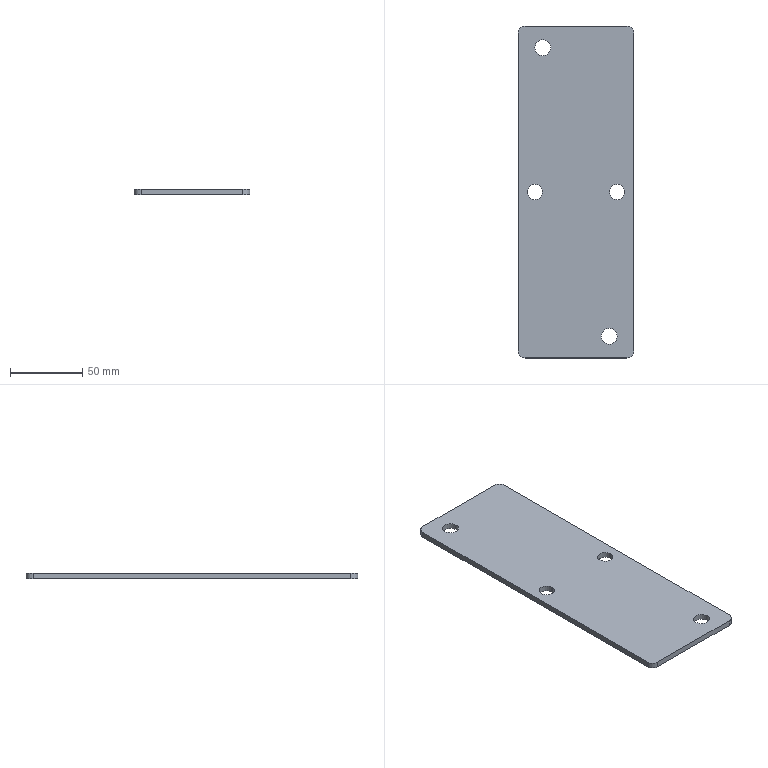Part | STEP file | 1_id78_x_t | 1 solid | 16 faces | box 80 x 230 x 4 mm | volume 72058 mm3 | cylinder 10 | plane 6 | commonest cylinder face diameters 10 x4 10.524 x4 11 x2
STEP:
#1=CARTESIAN_POINT('',(0.,0.,0.));
#2=DIRECTION('',(0.,0.,1.));
#3=DIRECTION('',(1.,0.,0.));
#4=AXIS2_PLACEMENT_3D('',#1,#2,#3);
#5=CARTESIAN_POINT('',(430.488,177.5,-105.));
#6=VERTEX_POINT('',#5);
#7=CARTESIAN_POINT('',(441.012,177.5,-105.));
#8=VERTEX_POINT('',#7);
#9=CARTESIAN_POINT('',(435.75,177.5,-105.));
#10=DIRECTION('',(0.,0.,1.));
#11=DIRECTION('',(1.,0.,0.));
#12=AXIS2_PLACEMENT_3D('',#9,#10,#11);
#13=CIRCLE('',#12,5.262);
#14=CARTESIAN_POINT('',(435.75,177.5,-101.));
#15=DIRECTION('',(0.,0.,1.));
#16=DIRECTION('',(1.,0.,0.));
#17=AXIS2_PLACEMENT_3D('',#14,#15,#16);
#18=CYLINDRICAL_SURFACE('',#17,5.262);
#19=CARTESIAN_POINT('',(0.,-4.));
#20=DIRECTION('',(1.,0.));
#21=VECTOR('',#20,1.);
#22=LINE('',#19,#21);
#23=(GEOMETRIC_REPRESENTATION_CONTEXT(2)PARAMETRIC_REPRESENTATION_CONTEXT()REPRESENTATION_CONTEXT('',''));
#24=DEFINITIONAL_REPRESENTATION('',(#22),#23);
#25=PCURVE('',#18,#24);
#26=CARTESIAN_POINT('',(272.727,177.5,-105.));
#27=DIRECTION('',(0.,0.,1.));
#28=DIRECTION('',(-1.,0.,0.));
#29=AXIS2_PLACEMENT_3D('',#26,#27,#28);
#30=PLANE('',#29);
#31=CARTESIAN_POINT('',(-163.023,-0.000000031));
#32=DIRECTION('',(-1.,0.));
#33=AXIS2_PLACEMENT_2D('',#31,#32);
#34=CIRCLE('',#33,5.262);
#35=(GEOMETRIC_REPRESENTATION_CONTEXT(2)PARAMETRIC_REPRESENTATION_CONTEXT()REPRESENTATION_CONTEXT('',''));
#36=DEFINITIONAL_REPRESENTATION('',(#34),#35);
#37=PCURVE('',#30,#36);
#38=SURFACE_CURVE('',#13,(#25,#37),.PCURVE_S1.);
#39=EDGE_CURVE('',#6,#8,#38,.T.);
#40=ORIENTED_EDGE('',*,*,#39,.T.);
#41=CARTESIAN_POINT('',(441.012,177.5,-101.));
#42=VERTEX_POINT('',#41);
#43=CARTESIAN_POINT('',(441.012,177.5,-101.));
#44=DIRECTION('',(0.,0.,1.));
#45=VECTOR('',#44,1.);
#46=LINE('',#43,#45);
#47=CARTESIAN_POINT('',(6.283,0.));
#48=DIRECTION('',(0.,1.));
#49=VECTOR('',#48,1.);
#50=LINE('',#47,#49);
#51=(GEOMETRIC_REPRESENTATION_CONTEXT(2)PARAMETRIC_REPRESENTATION_CONTEXT()REPRESENTATION_CONTEXT('',''));
#52=DEFINITIONAL_REPRESENTATION('',(#50),#51);
#53=PCURVE('',#18,#52);
#54=CARTESIAN_POINT('',(435.75,177.5,-101.));
#55=DIRECTION('',(0.,0.,1.));
#56=DIRECTION('',(1.,0.,0.));
#57=AXIS2_PLACEMENT_3D('',#54,#55,#56);
#58=CYLINDRICAL_SURFACE('',#57,5.262);
#59=CARTESIAN_POINT('',(0.000004723,0.));
#60=DIRECTION('',(0.,1.));
#61=VECTOR('',#60,1.);
#62=LINE('',#59,#61);
#63=(GEOMETRIC_REPRESENTATION_CONTEXT(2)PARAMETRIC_REPRESENTATION_CONTEXT()REPRESENTATION_CONTEXT('',''));
#64=DEFINITIONAL_REPRESENTATION('',(#62),#63);
#65=PCURVE('',#58,#64);
#66=SURFACE_CURVE('',#46,(#53,#65),.PCURVE_S1.);
#67=EDGE_CURVE('',#8,#42,#66,.T.);
#68=ORIENTED_EDGE('',*,*,#67,.T.);
#69=CARTESIAN_POINT('',(430.488,177.5,-101.));
#70=VERTEX_POINT('',#69);
#71=CARTESIAN_POINT('',(435.75,177.5,-101.));
#72=DIRECTION('',(0.,0.,1.));
#73=DIRECTION('',(1.,0.,0.));
#74=AXIS2_PLACEMENT_3D('',#71,#72,#73);
#75=CIRCLE('',#74,5.262);
#76=CARTESIAN_POINT('',(0.,0.));
#77=DIRECTION('',(1.,0.));
#78=VECTOR('',#77,1.);
#79=LINE('',#76,#78);
#80=(GEOMETRIC_REPRESENTATION_CONTEXT(2)PARAMETRIC_REPRESENTATION_CONTEXT()REPRESENTATION_CONTEXT('',''));
#81=DEFINITIONAL_REPRESENTATION('',(#79),#80);
#82=PCURVE('',#18,#81);
#83=CARTESIAN_POINT('',(272.727,177.5,-101.));
#84=DIRECTION('',(0.,0.,1.));
#85=DIRECTION('',(-1.,0.,0.));
#86=AXIS2_PLACEMENT_3D('',#83,#84,#85);
#87=PLANE('',#86);
#88=CARTESIAN_POINT('',(-163.023,-0.000000031));
#89=DIRECTION('',(-1.,0.));
#90=AXIS2_PLACEMENT_2D('',#88,#89);
#91=CIRCLE('',#90,5.262);
#92=(GEOMETRIC_REPRESENTATION_CONTEXT(2)PARAMETRIC_REPRESENTATION_CONTEXT()REPRESENTATION_CONTEXT('',''));
#93=DEFINITIONAL_REPRESENTATION('',(#91),#92);
#94=PCURVE('',#87,#93);
#95=SURFACE_CURVE('',#75,(#82,#94),.PCURVE_S1.);
#96=EDGE_CURVE('',#70,#42,#95,.T.);
#97=ORIENTED_EDGE('',*,*,#96,.F.);
#98=CARTESIAN_POINT('',(430.488,177.5,-101.));
#99=DIRECTION('',(0.,0.,-1.));
#100=VECTOR('',#99,1.);
#101=LINE('',#98,#100);
#102=CARTESIAN_POINT('',(3.142,0.));
#103=DIRECTION('',(0.,-1.));
#104=VECTOR('',#103,1.);
#105=LINE('',#102,#104);
#106=(GEOMETRIC_REPRESENTATION_CONTEXT(2)PARAMETRIC_REPRESENTATION_CONTEXT()REPRESENTATION_CONTEXT('',''));
#107=DEFINITIONAL_REPRESENTATION('',(#105),#106);
#108=PCURVE('',#18,#107);
#109=CARTESIAN_POINT('',(3.142,0.));
#110=DIRECTION('',(0.,-1.));
#111=VECTOR('',#110,1.);
#112=LINE('',#109,#111);
#113=(GEOMETRIC_REPRESENTATION_CONTEXT(2)PARAMETRIC_REPRESENTATION_CONTEXT()REPRESENTATION_CONTEXT('',''));
#114=DEFINITIONAL_REPRESENTATION('',(#112),#113);
#115=PCURVE('',#58,#114);
#116=SURFACE_CURVE('',#101,(#108,#115),.PCURVE_S1.);
#117=EDGE_CURVE('',#70,#6,#116,.T.);
#118=ORIENTED_EDGE('',*,*,#117,.T.);
#119=EDGE_LOOP('',(#40,#68,#97,#118));
#120=FACE_BOUND('',#119,.F.);
#121=ADVANCED_FACE('',(#120),#18,.F.);
#122=CARTESIAN_POINT('',(498.162,177.5,-105.));
#123=VERTEX_POINT('',#122);
#124=CARTESIAN_POINT('',(487.638,177.5,-105.));
#125=VERTEX_POINT('',#124);
#126=CARTESIAN_POINT('',(492.9,177.5,-105.));
#127=DIRECTION('',(0.,0.,1.));
#128=DIRECTION('',(1.,0.,0.));
#129=AXIS2_PLACEMENT_3D('',#126,#127,#128);
#130=CIRCLE('',#129,5.262);
#131=CARTESIAN_POINT('',(492.9,177.5,-101.));
#132=DIRECTION('',(0.,0.,1.));
#133=DIRECTION('',(1.,0.,0.));
#134=AXIS2_PLACEMENT_3D('',#131,#132,#133);
#135=CYLINDRICAL_SURFACE('',#134,5.262);
#136=CARTESIAN_POINT('',(0.,-4.));
#137=DIRECTION('',(1.,0.));
#138=VECTOR('',#137,1.);
#139=LINE('',#136,#138);
#140=(GEOMETRIC_REPRESENTATION_CONTEXT(2)PARAMETRIC_REPRESENTATION_CONTEXT()REPRESENTATION_CONTEXT('',''));
#141=DEFINITIONAL_REPRESENTATION('',(#139),#140);
#142=PCURVE('',#135,#141);
#143=CARTESIAN_POINT('',(-220.173,0.00003309));
#144=DIRECTION('',(-1.,0.));
#145=AXIS2_PLACEMENT_2D('',#143,#144);
#146=CIRCLE('',#145,5.262);
#147=(GEOMETRIC_REPRESENTATION_CONTEXT(2)PARAMETRIC_REPRESENTATION_CONTEXT()REPRESENTATION_CONTEXT('',''));
#148=DEFINITIONAL_REPRESENTATION('',(#146),#147);
#149=PCURVE('',#30,#148);
#150=SURFACE_CURVE('',#130,(#142,#149),.PCURVE_S1.);
#151=EDGE_CURVE('',#123,#125,#150,.T.);
#152=ORIENTED_EDGE('',*,*,#151,.T.);
#153=CARTESIAN_POINT('',(487.638,177.5,-101.));
#154=VERTEX_POINT('',#153);
#155=CARTESIAN_POINT('',(487.638,177.5,-101.));
#156=DIRECTION('',(0.,0.,1.));
#157=VECTOR('',#156,1.);
#158=LINE('',#155,#157);
#159=CARTESIAN_POINT('',(3.142,0.));
#160=DIRECTION('',(0.,1.));
#161=VECTOR('',#160,1.);
#162=LINE('',#159,#161);
#163=(GEOMETRIC_REPRESENTATION_CONTEXT(2)PARAMETRIC_REPRESENTATION_CONTEXT()REPRESENTATION_CONTEXT('',''));
#164=DEFINITIONAL_REPRESENTATION('',(#162),#163);
#165=PCURVE('',#135,#164);
#166=CARTESIAN_POINT('',(492.9,177.5,-101.));
#167=DIRECTION('',(0.,0.,1.));
#168=DIRECTION('',(1.,0.,0.));
#169=AXIS2_PLACEMENT_3D('',#166,#167,#168);
#170=CYLINDRICAL_SURFACE('',#169,5.262);
#171=CARTESIAN_POINT('',(3.142,0.));
#172=DIRECTION('',(0.,1.));
#173=VECTOR('',#172,1.);
#174=LINE('',#171,#173);
#175=(GEOMETRIC_REPRESENTATION_CONTEXT(2)PARAMETRIC_REPRESENTATION_CONTEXT()REPRESENTATION_CONTEXT('',''));
#176=DEFINITIONAL_REPRESENTATION('',(#174),#175);
#177=PCURVE('',#170,#176);
#178=SURFACE_CURVE('',#158,(#165,#177),.PCURVE_S1.);
#179=EDGE_CURVE('',#125,#154,#178,.T.);
#180=ORIENTED_EDGE('',*,*,#179,.T.);
#181=CARTESIAN_POINT('',(498.162,177.5,-101.));
#182=VERTEX_POINT('',#181);
#183=CARTESIAN_POINT('',(492.9,177.5,-101.));
#184=DIRECTION('',(0.,0.,1.));
#185=DIRECTION('',(1.,0.,0.));
#186=AXIS2_PLACEMENT_3D('',#183,#184,#185);
#187=CIRCLE('',#186,5.262);
#188=CARTESIAN_POINT('',(0.,0.));
#189=DIRECTION('',(1.,0.));
#190=VECTOR('',#189,1.);
#191=LINE('',#188,#190);
#192=(GEOMETRIC_REPRESENTATION_CONTEXT(2)PARAMETRIC_REPRESENTATION_CONTEXT()REPRESENTATION_CONTEXT('',''));
#193=DEFINITIONAL_REPRESENTATION('',(#191),#192);
#194=PCURVE('',#135,#193);
#195=CARTESIAN_POINT('',(-220.173,0.00003309));
#196=DIRECTION('',(-1.,0.));
#197=AXIS2_PLACEMENT_2D('',#195,#196);
#198=CIRCLE('',#197,5.262);
#199=(GEOMETRIC_REPRESENTATION_CONTEXT(2)PARAMETRIC_REPRESENTATION_CONTEXT()REPRESENTATION_CONTEXT('',''));
#200=DEFINITIONAL_REPRESENTATION('',(#198),#199);
#201=PCURVE('',#87,#200);
#202=SURFACE_CURVE('',#187,(#194,#201),.PCURVE_S1.);
#203=EDGE_CURVE('',#182,#154,#202,.T.);
#204=ORIENTED_EDGE('',*,*,#203,.F.);
#205=CARTESIAN_POINT('',(498.162,177.5,-101.));
#206=DIRECTION('',(0.,0.,-1.));
#207=VECTOR('',#206,1.);
#208=LINE('',#205,#207);
#209=CARTESIAN_POINT('',(0.000004723,0.));
#210=DIRECTION('',(0.,-1.));
#211=VECTOR('',#210,1.);
#212=LINE('',#209,#211);
#213=(GEOMETRIC_REPRESENTATION_CONTEXT(2)PARAMETRIC_REPRESENTATION_CONTEXT()REPRESENTATION_CONTEXT('',''));
#214=DEFINITIONAL_REPRESENTATION('',(#212),#213);
#215=PCURVE('',#135,#214);
#216=CARTESIAN_POINT('',(6.283,0.));
#217=DIRECTION('',(0.,-1.));
#218=VECTOR('',#217,1.);
#219=LINE('',#216,#218);
#220=(GEOMETRIC_REPRESENTATION_CONTEXT(2)PARAMETRIC_REPRESENTATION_CONTEXT()REPRESENTATION_CONTEXT('',''));
#221=DEFINITIONAL_REPRESENTATION('',(#219),#220);
#222=PCURVE('',#170,#221);
#223=SURFACE_CURVE('',#208,(#215,#222),.PCURVE_S1.);
#224=EDGE_CURVE('',#182,#123,#223,.T.);
#225=ORIENTED_EDGE('',*,*,#224,.T.);
#226=EDGE_LOOP('',(#152,#180,#204,#225));
#227=FACE_BOUND('',#226,.F.);
#228=ADVANCED_FACE('',(#227),#135,.F.);
#229=CARTESIAN_POINT('',(499.325,292.5,-101.));
#230=VERTEX_POINT('',#229);
#231=CARTESIAN_POINT('',(499.325,292.5,-105.));
#232=VERTEX_POINT('',#231);
#233=CARTESIAN_POINT('',(499.325,292.5,-101.));
#234=DIRECTION('',(0.,0.,-1.));
#235=VECTOR('',#234,1.);
#236=LINE('',#233,#235);
#237=CARTESIAN_POINT('',(499.325,287.5,-101.));
#238=DIRECTION('',(0.,0.,-1.));
#239=DIRECTION('',(-1.,0.,0.));
#240=AXIS2_PLACEMENT_3D('',#237,#238,#239);
#241=CYLINDRICAL_SURFACE('',#240,5.);
#242=CARTESIAN_POINT('',(1.571,0.));
#243=DIRECTION('',(0.,1.));
#244=VECTOR('',#243,1.);
#245=LINE('',#242,#244);
#246=(GEOMETRIC_REPRESENTATION_CONTEXT(2)PARAMETRIC_REPRESENTATION_CONTEXT()REPRESENTATION_CONTEXT('',''));
#247=DEFINITIONAL_REPRESENTATION('',(#245),#246);
#248=PCURVE('',#241,#247);
#249=CARTESIAN_POINT('',(272.727,292.5,-101.));
#250=DIRECTION('',(0.,1.,0.));
#251=DIRECTION('',(-1.,0.,0.));
#252=AXIS2_PLACEMENT_3D('',#249,#250,#251);
#253=PLANE('',#252);
#254=CARTESIAN_POINT('',(-226.598,0.));
#255=DIRECTION('',(0.,-1.));
#256=VECTOR('',#255,1.);
#257=LINE('',#254,#256);
#258=(GEOMETRIC_REPRESENTATION_CONTEXT(2)PARAMETRIC_REPRESENTATION_CONTEXT()REPRESENTATION_CONTEXT('',''));
#259=DEFINITIONAL_REPRESENTATION('',(#257),#258);
#260=PCURVE('',#253,#259);
#261=SURFACE_CURVE('',#236,(#248,#260),.PCURVE_S1.);
#262=EDGE_CURVE('',#230,#232,#261,.T.);
#263=ORIENTED_EDGE('',*,*,#262,.F.);
#264=CARTESIAN_POINT('',(504.325,287.5,-101.));
#265=VERTEX_POINT('',#264);
#266=CARTESIAN_POINT('',(499.325,287.5,-101.));
#267=DIRECTION('',(0.,0.,-1.));
#268=DIRECTION('',(-1.,0.,0.));
#269=AXIS2_PLACEMENT_3D('',#266,#267,#268);
#270=CIRCLE('',#269,5.);
#271=CARTESIAN_POINT('',(0.,0.));
#272=DIRECTION('',(1.,0.));
#273=VECTOR('',#272,1.);
#274=LINE('',#271,#273);
#275=(GEOMETRIC_REPRESENTATION_CONTEXT(2)PARAMETRIC_REPRESENTATION_CONTEXT()REPRESENTATION_CONTEXT('',''));
#276=DEFINITIONAL_REPRESENTATION('',(#274),#275);
#277=PCURVE('',#241,#276);
#278=CARTESIAN_POINT('',(-221.598,-110.));
#279=CARTESIAN_POINT('',(-221.598,-118.66));
#280=CARTESIAN_POINT('',(-229.098,-114.33));
#281=CARTESIAN_POINT('',(-236.598,-110.));
#282=CARTESIAN_POINT('',(-229.098,-105.67));
#283=CARTESIAN_POINT('',(-221.598,-101.34));
#284=CARTESIAN_POINT('',(-221.598,-110.));
#285=(BOUNDED_CURVE()B_SPLINE_CURVE(2,(#278,#279,#280,#281,#282,#283,#284),.UNSPECIFIED.,.T.,.F.)B_SPLINE_CURVE_WITH_KNOTS((1,2,2,2,2,1),(-2.094,0.,2.094,4.189,6.283,8.378),.UNSPECIFIED.)CURVE()GEOMETRIC_REPRESENTATION_ITEM()RATIONAL_B_SPLINE_CURVE((1.,0.5,1.,0.5,1.,0.5,1.))REPRESENTATION_ITEM(''));
#286=(GEOMETRIC_REPRESENTATION_CONTEXT(2)PARAMETRIC_REPRESENTATION_CONTEXT()REPRESENTATION_CONTEXT('',''));
#287=DEFINITIONAL_REPRESENTATION('',(#285),#286);
#288=PCURVE('',#87,#287);
#289=SURFACE_CURVE('',#270,(#277,#288),.PCURVE_S1.);
#290=EDGE_CURVE('',#230,#265,#289,.T.);
#291=ORIENTED_EDGE('',*,*,#290,.T.);
#292=CARTESIAN_POINT('',(504.325,287.5,-105.));
#293=VERTEX_POINT('',#292);
#294=CARTESIAN_POINT('',(504.325,287.5,-101.));
#295=DIRECTION('',(0.,0.,-1.));
#296=VECTOR('',#295,1.);
#297=LINE('',#294,#296);
#298=CARTESIAN_POINT('',(3.142,0.));
#299=DIRECTION('',(0.,1.));
#300=VECTOR('',#299,1.);
#301=LINE('',#298,#300);
#302=(GEOMETRIC_REPRESENTATION_CONTEXT(2)PARAMETRIC_REPRESENTATION_CONTEXT()REPRESENTATION_CONTEXT('',''));
#303=DEFINITIONAL_REPRESENTATION('',(#301),#302);
#304=PCURVE('',#241,#303);
#305=CARTESIAN_POINT('',(504.325,177.5,-101.));
#306=DIRECTION('',(-1.,0.,0.));
#307=DIRECTION('',(0.,-1.,0.));
#308=AXIS2_PLACEMENT_3D('',#305,#306,#307);
#309=PLANE('',#308);
#310=CARTESIAN_POINT('',(-110.,0.));
#311=DIRECTION('',(0.,-1.));
#312=VECTOR('',#311,1.);
#313=LINE('',#310,#312);
#314=(GEOMETRIC_REPRESENTATION_CONTEXT(2)PARAMETRIC_REPRESENTATION_CONTEXT()REPRESENTATION_CONTEXT('',''));
#315=DEFINITIONAL_REPRESENTATION('',(#313),#314);
#316=PCURVE('',#309,#315);
#317=SURFACE_CURVE('',#297,(#304,#316),.PCURVE_S1.);
#318=EDGE_CURVE('',#265,#293,#317,.T.);
#319=ORIENTED_EDGE('',*,*,#318,.T.);
#320=CARTESIAN_POINT('',(499.325,287.5,-105.));
#321=DIRECTION('',(0.,0.,-1.));
#322=DIRECTION('',(-1.,0.,0.));
#323=AXIS2_PLACEMENT_3D('',#320,#321,#322);
#324=CIRCLE('',#323,5.);
#325=CARTESIAN_POINT('',(0.,4.));
#326=DIRECTION('',(1.,0.));
#327=VECTOR('',#326,1.);
#328=LINE('',#325,#327);
#329=(GEOMETRIC_REPRESENTATION_CONTEXT(2)PARAMETRIC_REPRESENTATION_CONTEXT()REPRESENTATION_CONTEXT('',''));
#330=DEFINITIONAL_REPRESENTATION('',(#328),#329);
#331=PCURVE('',#241,#330);
#332=CARTESIAN_POINT('',(-221.598,-110.));
#333=CARTESIAN_POINT('',(-221.598,-118.66));
#334=CARTESIAN_POINT('',(-229.098,-114.33));
#335=CARTESIAN_POINT('',(-236.598,-110.));
#336=CARTESIAN_POINT('',(-229.098,-105.67));
#337=CARTESIAN_POINT('',(-221.598,-101.34));
#338=CARTESIAN_POINT('',(-221.598,-110.));
#339=(BOUNDED_CURVE()B_SPLINE_CURVE(2,(#332,#333,#334,#335,#336,#337,#338),.UNSPECIFIED.,.T.,.F.)B_SPLINE_CURVE_WITH_KNOTS((1,2,2,2,2,1),(-2.094,0.,2.094,4.189,6.283,8.378),.UNSPECIFIED.)CURVE()GEOMETRIC_REPRESENTATION_ITEM()RATIONAL_B_SPLINE_CURVE((1.,0.5,1.,0.5,1.,0.5,1.))REPRESENTATION_ITEM(''));
#340=(GEOMETRIC_REPRESENTATION_CONTEXT(2)PARAMETRIC_REPRESENTATION_CONTEXT()REPRESENTATION_CONTEXT('',''));
#341=DEFINITIONAL_REPRESENTATION('',(#339),#340);
#342=PCURVE('',#30,#341);
#343=SURFACE_CURVE('',#324,(#331,#342),.PCURVE_S1.);
#344=EDGE_CURVE('',#232,#293,#343,.T.);
#345=ORIENTED_EDGE('',*,*,#344,.F.);
#346=EDGE_LOOP('',(#263,#291,#319,#345));
#347=FACE_BOUND('',#346,.T.);
#348=ADVANCED_FACE('',(#347),#241,.T.);
#349=ORIENTED_EDGE('',*,*,#318,.F.);
#350=CARTESIAN_POINT('',(504.325,67.5,-101.));
#351=VERTEX_POINT('',#350);
#352=CARTESIAN_POINT('',(504.325,177.5,-101.));
#353=DIRECTION('',(0.,1.,0.));
#354=VECTOR('',#353,1.);
#355=LINE('',#352,#354);
#356=CARTESIAN_POINT('',(0.,0.));
#357=DIRECTION('',(-1.,0.));
#358=VECTOR('',#357,1.);
#359=LINE('',#356,#358);
#360=(GEOMETRIC_REPRESENTATION_CONTEXT(2)PARAMETRIC_REPRESENTATION_CONTEXT()REPRESENTATION_CONTEXT('',''));
#361=DEFINITIONAL_REPRESENTATION('',(#359),#360);
#362=PCURVE('',#309,#361);
#363=CARTESIAN_POINT('',(-231.598,0.));
#364=DIRECTION('',(0.,-1.));
#365=VECTOR('',#364,1.);
#366=LINE('',#363,#365);
#367=(GEOMETRIC_REPRESENTATION_CONTEXT(2)PARAMETRIC_REPRESENTATION_CONTEXT()REPRESENTATION_CONTEXT('',''));
#368=DEFINITIONAL_REPRESENTATION('',(#366),#367);
#369=PCURVE('',#87,#368);
#370=SURFACE_CURVE('',#355,(#362,#369),.PCURVE_S1.);
#371=EDGE_CURVE('',#351,#265,#370,.T.);
#372=ORIENTED_EDGE('',*,*,#371,.F.);
#373=CARTESIAN_POINT('',(504.325,67.5,-105.));
#374=VERTEX_POINT('',#373);
#375=CARTESIAN_POINT('',(504.325,67.5,-101.));
#376=DIRECTION('',(0.,0.,-1.));
#377=VECTOR('',#376,1.);
#378=LINE('',#375,#377);
#379=CARTESIAN_POINT('',(110.,0.));
#380=DIRECTION('',(0.,-1.));
#381=VECTOR('',#380,1.);
#382=LINE('',#379,#381);
#383=(GEOMETRIC_REPRESENTATION_CONTEXT(2)PARAMETRIC_REPRESENTATION_CONTEXT()REPRESENTATION_CONTEXT('',''));
#384=DEFINITIONAL_REPRESENTATION('',(#382),#383);
#385=PCURVE('',#309,#384);
#386=CARTESIAN_POINT('',(499.325,67.5,-101.));
#387=DIRECTION('',(0.,0.,-1.));
#388=DIRECTION('',(-1.,0.,0.));
#389=AXIS2_PLACEMENT_3D('',#386,#387,#388);
#390=CYLINDRICAL_SURFACE('',#389,5.);
#391=CARTESIAN_POINT('',(3.142,0.));
#392=DIRECTION('',(0.,1.));
#393=VECTOR('',#392,1.);
#394=LINE('',#391,#393);
#395=(GEOMETRIC_REPRESENTATION_CONTEXT(2)PARAMETRIC_REPRESENTATION_CONTEXT()REPRESENTATION_CONTEXT('',''));
#396=DEFINITIONAL_REPRESENTATION('',(#394),#395);
#397=PCURVE('',#390,#396);
#398=SURFACE_CURVE('',#378,(#385,#397),.PCURVE_S1.);
#399=EDGE_CURVE('',#351,#374,#398,.T.);
#400=ORIENTED_EDGE('',*,*,#399,.T.);
#401=CARTESIAN_POINT('',(504.325,177.5,-105.));
#402=DIRECTION('',(0.,1.,0.));
#403=VECTOR('',#402,1.);
#404=LINE('',#401,#403);
#405=CARTESIAN_POINT('',(0.,-4.));
#406=DIRECTION('',(-1.,0.));
#407=VECTOR('',#406,1.);
#408=LINE('',#405,#407);
#409=(GEOMETRIC_REPRESENTATION_CONTEXT(2)PARAMETRIC_REPRESENTATION_CONTEXT()REPRESENTATION_CONTEXT('',''));
#410=DEFINITIONAL_REPRESENTATION('',(#408),#409);
#411=PCURVE('',#309,#410);
#412=CARTESIAN_POINT('',(-231.598,0.));
#413=DIRECTION('',(0.,-1.));
#414=VECTOR('',#413,1.);
#415=LINE('',#412,#414);
#416=(GEOMETRIC_REPRESENTATION_CONTEXT(2)PARAMETRIC_REPRESENTATION_CONTEXT()REPRESENTATION_CONTEXT('',''));
#417=DEFINITIONAL_REPRESENTATION('',(#415),#416);
#418=PCURVE('',#30,#417);
#419=SURFACE_CURVE('',#404,(#411,#418),.PCURVE_S1.);
#420=EDGE_CURVE('',#374,#293,#419,.T.);
#421=ORIENTED_EDGE('',*,*,#420,.T.);
#422=EDGE_LOOP('',(#349,#372,#400,#421));
#423=FACE_BOUND('',#422,.T.);
#424=ADVANCED_FACE('',(#423),#309,.F.);
#425=ORIENTED_EDGE('',*,*,#399,.F.);
#426=CARTESIAN_POINT('',(499.325,62.5,-101.));
#427=VERTEX_POINT('',#426);
#428=CARTESIAN_POINT('',(499.325,67.5,-101.));
#429=DIRECTION('',(0.,0.,-1.));
#430=DIRECTION('',(-1.,0.,0.));
#431=AXIS2_PLACEMENT_3D('',#428,#429,#430);
#432=CIRCLE('',#431,5.);
#433=CARTESIAN_POINT('',(0.,0.));
#434=DIRECTION('',(1.,0.));
#435=VECTOR('',#434,1.);
#436=LINE('',#433,#435);
#437=(GEOMETRIC_REPRESENTATION_CONTEXT(2)PARAMETRIC_REPRESENTATION_CONTEXT()REPRESENTATION_CONTEXT('',''));
#438=DEFINITIONAL_REPRESENTATION('',(#436),#437);
#439=PCURVE('',#390,#438);
#440=CARTESIAN_POINT('',(-221.598,110.));
#441=CARTESIAN_POINT('',(-221.598,101.34));
#442=CARTESIAN_POINT('',(-229.098,105.67));
#443=CARTESIAN_POINT('',(-236.598,110.));
#444=CARTESIAN_POINT('',(-229.098,114.33));
#445=CARTESIAN_POINT('',(-221.598,118.66));
#446=CARTESIAN_POINT('',(-221.598,110.));
#447=(BOUNDED_CURVE()B_SPLINE_CURVE(2,(#440,#441,#442,#443,#444,#445,#446),.UNSPECIFIED.,.T.,.F.)B_SPLINE_CURVE_WITH_KNOTS((1,2,2,2,2,1),(-2.094,0.,2.094,4.189,6.283,8.378),.UNSPECIFIED.)CURVE()GEOMETRIC_REPRESENTATION_ITEM()RATIONAL_B_SPLINE_CURVE((1.,0.5,1.,0.5,1.,0.5,1.))REPRESENTATION_ITEM(''));
#448=(GEOMETRIC_REPRESENTATION_CONTEXT(2)PARAMETRIC_REPRESENTATION_CONTEXT()REPRESENTATION_CONTEXT('',''));
#449=DEFINITIONAL_REPRESENTATION('',(#447),#448);
#450=PCURVE('',#87,#449);
#451=SURFACE_CURVE('',#432,(#439,#450),.PCURVE_S1.);
#452=EDGE_CURVE('',#351,#427,#451,.T.);
#453=ORIENTED_EDGE('',*,*,#452,.T.);
#454=CARTESIAN_POINT('',(499.325,62.5,-105.));
#455=VERTEX_POINT('',#454);
#456=CARTESIAN_POINT('',(499.325,62.5,-101.));
#457=DIRECTION('',(0.,0.,-1.));
#458=VECTOR('',#457,1.);
#459=LINE('',#456,#458);
#460=CARTESIAN_POINT('',(4.712,0.));
#461=DIRECTION('',(0.,1.));
#462=VECTOR('',#461,1.);
#463=LINE('',#460,#462);
#464=(GEOMETRIC_REPRESENTATION_CONTEXT(2)PARAMETRIC_REPRESENTATION_CONTEXT()REPRESENTATION_CONTEXT('',''));
#465=DEFINITIONAL_REPRESENTATION('',(#463),#464);
#466=PCURVE('',#390,#465);
#467=CARTESIAN_POINT('',(272.727,62.5,-101.));
#468=DIRECTION('',(0.,1.,0.));
#469=DIRECTION('',(-1.,0.,0.));
#470=AXIS2_PLACEMENT_3D('',#467,#468,#469);
#471=PLANE('',#470);
#472=CARTESIAN_POINT('',(-226.598,0.));
#473=DIRECTION('',(0.,-1.));
#474=VECTOR('',#473,1.);
#475=LINE('',#472,#474);
#476=(GEOMETRIC_REPRESENTATION_CONTEXT(2)PARAMETRIC_REPRESENTATION_CONTEXT()REPRESENTATION_CONTEXT('',''));
#477=DEFINITIONAL_REPRESENTATION('',(#475),#476);
#478=PCURVE('',#471,#477);
#479=SURFACE_CURVE('',#459,(#466,#478),.PCURVE_S1.);
#480=EDGE_CURVE('',#427,#455,#479,.T.);
#481=ORIENTED_EDGE('',*,*,#480,.T.);
#482=CARTESIAN_POINT('',(499.325,67.5,-105.));
#483=DIRECTION('',(0.,0.,-1.));
#484=DIRECTION('',(-1.,0.,0.));
#485=AXIS2_PLACEMENT_3D('',#482,#483,#484);
#486=CIRCLE('',#485,5.);
#487=CARTESIAN_POINT('',(0.,4.));
#488=DIRECTION('',(1.,0.));
#489=VECTOR('',#488,1.);
#490=LINE('',#487,#489);
#491=(GEOMETRIC_REPRESENTATION_CONTEXT(2)PARAMETRIC_REPRESENTATION_CONTEXT()REPRESENTATION_CONTEXT('',''));
#492=DEFINITIONAL_REPRESENTATION('',(#490),#491);
#493=PCURVE('',#390,#492);
#494=CARTESIAN_POINT('',(-221.598,110.));
#495=CARTESIAN_POINT('',(-221.598,101.34));
#496=CARTESIAN_POINT('',(-229.098,105.67));
#497=CARTESIAN_POINT('',(-236.598,110.));
#498=CARTESIAN_POINT('',(-229.098,114.33));
#499=CARTESIAN_POINT('',(-221.598,118.66));
#500=CARTESIAN_POINT('',(-221.598,110.));
#501=(BOUNDED_CURVE()B_SPLINE_CURVE(2,(#494,#495,#496,#497,#498,#499,#500),.UNSPECIFIED.,.T.,.F.)B_SPLINE_CURVE_WITH_KNOTS((1,2,2,2,2,1),(-2.094,0.,2.094,4.189,6.283,8.378),.UNSPECIFIED.)CURVE()GEOMETRIC_REPRESENTATION_ITEM()RATIONAL_B_SPLINE_CURVE((1.,0.5,1.,0.5,1.,0.5,1.))REPRESENTATION_ITEM(''));
#502=(GEOMETRIC_REPRESENTATION_CONTEXT(2)PARAMETRIC_REPRESENTATION_CONTEXT()REPRESENTATION_CONTEXT('',''));
#503=DEFINITIONAL_REPRESENTATION('',(#501),#502);
#504=PCURVE('',#30,#503);
#505=SURFACE_CURVE('',#486,(#493,#504),.PCURVE_S1.);
#506=EDGE_CURVE('',#374,#455,#505,.T.);
#507=ORIENTED_EDGE('',*,*,#506,.F.);
#508=EDGE_LOOP('',(#425,#453,#481,#507));
#509=FACE_BOUND('',#508,.T.);
#510=ADVANCED_FACE('',(#509),#390,.T.);
#511=ORIENTED_EDGE('',*,*,#480,.F.);
#512=CARTESIAN_POINT('',(429.325,62.5,-101.));
#513=VERTEX_POINT('',#512);
#514=CARTESIAN_POINT('',(272.727,62.5,-101.));
#515=DIRECTION('',(1.,0.,0.));
#516=VECTOR('',#515,1.);
#517=LINE('',#514,#516);
#518=CARTESIAN_POINT('',(0.,0.));
#519=DIRECTION('',(-1.,0.));
#520=VECTOR('',#519,1.);
#521=LINE('',#518,#520);
#522=(GEOMETRIC_REPRESENTATION_CONTEXT(2)PARAMETRIC_REPRESENTATION_CONTEXT()REPRESENTATION_CONTEXT('',''));
#523=DEFINITIONAL_REPRESENTATION('',(#521),#522);
#524=PCURVE('',#471,#523);
#525=CARTESIAN_POINT('',(0.,115.));
#526=DIRECTION('',(-1.,0.));
#527=VECTOR('',#526,1.);
#528=LINE('',#525,#527);
#529=(GEOMETRIC_REPRESENTATION_CONTEXT(2)PARAMETRIC_REPRESENTATION_CONTEXT()REPRESENTATION_CONTEXT('',''));
#530=DEFINITIONAL_REPRESENTATION('',(#528),#529);
#531=PCURVE('',#87,#530);
#532=SURFACE_CURVE('',#517,(#524,#531),.PCURVE_S1.);
#533=EDGE_CURVE('',#513,#427,#532,.T.);
#534=ORIENTED_EDGE('',*,*,#533,.F.);
#535=CARTESIAN_POINT('',(429.325,62.5,-105.));
#536=VERTEX_POINT('',#535);
#537=CARTESIAN_POINT('',(429.325,62.5,-101.));
#538=DIRECTION('',(0.,0.,-1.));
#539=VECTOR('',#538,1.);
#540=LINE('',#537,#539);
#541=CARTESIAN_POINT('',(-156.598,0.));
#542=DIRECTION('',(0.,-1.));
#543=VECTOR('',#542,1.);
#544=LINE('',#541,#543);
#545=(GEOMETRIC_REPRESENTATION_CONTEXT(2)PARAMETRIC_REPRESENTATION_CONTEXT()REPRESENTATION_CONTEXT('',''));
#546=DEFINITIONAL_REPRESENTATION('',(#544),#545);
#547=PCURVE('',#471,#546);
#548=CARTESIAN_POINT('',(429.325,67.5,-101.));
#549=DIRECTION('',(0.,0.,-1.));
#550=DIRECTION('',(-1.,0.,0.));
#551=AXIS2_PLACEMENT_3D('',#548,#549,#550);
#552=CYLINDRICAL_SURFACE('',#551,5.);
#553=CARTESIAN_POINT('',(4.712,0.));
#554=DIRECTION('',(0.,1.));
#555=VECTOR('',#554,1.);
#556=LINE('',#553,#555);
#557=(GEOMETRIC_REPRESENTATION_CONTEXT(2)PARAMETRIC_REPRESENTATION_CONTEXT()REPRESENTATION_CONTEXT('',''));
#558=DEFINITIONAL_REPRESENTATION('',(#556),#557);
#559=PCURVE('',#552,#558);
#560=SURFACE_CURVE('',#540,(#547,#559),.PCURVE_S1.);
#561=EDGE_CURVE('',#513,#536,#560,.T.);
#562=ORIENTED_EDGE('',*,*,#561,.T.);
#563=CARTESIAN_POINT('',(272.727,62.5,-105.));
#564=DIRECTION('',(1.,0.,0.));
#565=VECTOR('',#564,1.);
#566=LINE('',#563,#565);
#567=CARTESIAN_POINT('',(0.,-4.));
#568=DIRECTION('',(-1.,0.));
#569=VECTOR('',#568,1.);
#570=LINE('',#567,#569);
#571=(GEOMETRIC_REPRESENTATION_CONTEXT(2)PARAMETRIC_REPRESENTATION_CONTEXT()REPRESENTATION_CONTEXT('',''));
#572=DEFINITIONAL_REPRESENTATION('',(#570),#571);
#573=PCURVE('',#471,#572);
#574=CARTESIAN_POINT('',(0.,115.));
#575=DIRECTION('',(-1.,0.));
#576=VECTOR('',#575,1.);
#577=LINE('',#574,#576);
#578=(GEOMETRIC_REPRESENTATION_CONTEXT(2)PARAMETRIC_REPRESENTATION_CONTEXT()REPRESENTATION_CONTEXT('',''));
#579=DEFINITIONAL_REPRESENTATION('',(#577),#578);
#580=PCURVE('',#30,#579);
#581=SURFACE_CURVE('',#566,(#573,#580),.PCURVE_S1.);
#582=EDGE_CURVE('',#536,#455,#581,.T.);
#583=ORIENTED_EDGE('',*,*,#582,.T.);
#584=EDGE_LOOP('',(#511,#534,#562,#583));
#585=FACE_BOUND('',#584,.T.);
#586=ADVANCED_FACE('',(#585),#471,.F.);
#587=ORIENTED_EDGE('',*,*,#561,.F.);
#588=CARTESIAN_POINT('',(424.325,67.5,-101.));
#589=VERTEX_POINT('',#588);
#590=CARTESIAN_POINT('',(429.325,67.5,-101.));
#591=DIRECTION('',(0.,0.,-1.));
#592=DIRECTION('',(-1.,0.,0.));
#593=AXIS2_PLACEMENT_3D('',#590,#591,#592);
#594=CIRCLE('',#593,5.);
#595=CARTESIAN_POINT('',(0.,0.));
#596=DIRECTION('',(1.,0.));
#597=VECTOR('',#596,1.);
#598=LINE('',#595,#597);
#599=(GEOMETRIC_REPRESENTATION_CONTEXT(2)PARAMETRIC_REPRESENTATION_CONTEXT()REPRESENTATION_CONTEXT('',''));
#600=DEFINITIONAL_REPRESENTATION('',(#598),#599);
#601=PCURVE('',#552,#600);
#602=CARTESIAN_POINT('',(-151.598,110.));
#603=CARTESIAN_POINT('',(-151.598,101.34));
#604=CARTESIAN_POINT('',(-159.098,105.67));
#605=CARTESIAN_POINT('',(-166.598,110.));
#606=CARTESIAN_POINT('',(-159.098,114.33));
#607=CARTESIAN_POINT('',(-151.598,118.66));
#608=CARTESIAN_POINT('',(-151.598,110.));
#609=(BOUNDED_CURVE()B_SPLINE_CURVE(2,(#602,#603,#604,#605,#606,#607,#608),.UNSPECIFIED.,.T.,.F.)B_SPLINE_CURVE_WITH_KNOTS((1,2,2,2,2,1),(-2.094,0.,2.094,4.189,6.283,8.378),.UNSPECIFIED.)CURVE()GEOMETRIC_REPRESENTATION_ITEM()RATIONAL_B_SPLINE_CURVE((1.,0.5,1.,0.5,1.,0.5,1.))REPRESENTATION_ITEM(''));
#610=(GEOMETRIC_REPRESENTATION_CONTEXT(2)PARAMETRIC_REPRESENTATION_CONTEXT()REPRESENTATION_CONTEXT('',''));
#611=DEFINITIONAL_REPRESENTATION('',(#609),#610);
#612=PCURVE('',#87,#611);
#613=SURFACE_CURVE('',#594,(#601,#612),.PCURVE_S1.);
#614=EDGE_CURVE('',#513,#589,#613,.T.);
#615=ORIENTED_EDGE('',*,*,#614,.T.);
#616=CARTESIAN_POINT('',(424.325,67.5,-105.));
#617=VERTEX_POINT('',#616);
#618=CARTESIAN_POINT('',(424.325,67.5,-101.));
#619=DIRECTION('',(0.,0.,-1.));
#620=VECTOR('',#619,1.);
#621=LINE('',#618,#620);
#622=CARTESIAN_POINT('',(6.283,0.));
#623=DIRECTION('',(0.,1.));
#624=VECTOR('',#623,1.);
#625=LINE('',#622,#624);
#626=(GEOMETRIC_REPRESENTATION_CONTEXT(2)PARAMETRIC_REPRESENTATION_CONTEXT()REPRESENTATION_CONTEXT('',''));
#627=DEFINITIONAL_REPRESENTATION('',(#625),#626);
#628=PCURVE('',#552,#627);
#629=CARTESIAN_POINT('',(424.325,177.5,-101.));
#630=DIRECTION('',(-1.,0.,0.));
#631=DIRECTION('',(0.,-1.,0.));
#632=AXIS2_PLACEMENT_3D('',#629,#630,#631);
#633=PLANE('',#632);
#634=CARTESIAN_POINT('',(110.,0.));
#635=DIRECTION('',(0.,-1.));
#636=VECTOR('',#635,1.);
#637=LINE('',#634,#636);
#638=(GEOMETRIC_REPRESENTATION_CONTEXT(2)PARAMETRIC_REPRESENTATION_CONTEXT()REPRESENTATION_CONTEXT('',''));
#639=DEFINITIONAL_REPRESENTATION('',(#637),#638);
#640=PCURVE('',#633,#639);
#641=SURFACE_CURVE('',#621,(#628,#640),.PCURVE_S1.);
#642=EDGE_CURVE('',#589,#617,#641,.T.);
#643=ORIENTED_EDGE('',*,*,#642,.T.);
#644=CARTESIAN_POINT('',(429.325,67.5,-105.));
#645=DIRECTION('',(0.,0.,-1.));
#646=DIRECTION('',(-1.,0.,0.));
#647=AXIS2_PLACEMENT_3D('',#644,#645,#646);
#648=CIRCLE('',#647,5.);
#649=CARTESIAN_POINT('',(0.,4.));
#650=DIRECTION('',(1.,0.));
#651=VECTOR('',#650,1.);
#652=LINE('',#649,#651);
#653=(GEOMETRIC_REPRESENTATION_CONTEXT(2)PARAMETRIC_REPRESENTATION_CONTEXT()REPRESENTATION_CONTEXT('',''));
#654=DEFINITIONAL_REPRESENTATION('',(#652),#653);
#655=PCURVE('',#552,#654);
#656=CARTESIAN_POINT('',(-151.598,110.));
#657=CARTESIAN_POINT('',(-151.598,101.34));
#658=CARTESIAN_POINT('',(-159.098,105.67));
#659=CARTESIAN_POINT('',(-166.598,110.));
#660=CARTESIAN_POINT('',(-159.098,114.33));
#661=CARTESIAN_POINT('',(-151.598,118.66));
#662=CARTESIAN_POINT('',(-151.598,110.));
#663=(BOUNDED_CURVE()B_SPLINE_CURVE(2,(#656,#657,#658,#659,#660,#661,#662),.UNSPECIFIED.,.T.,.F.)B_SPLINE_CURVE_WITH_KNOTS((1,2,2,2,2,1),(-2.094,0.,2.094,4.189,6.283,8.378),.UNSPECIFIED.)CURVE()GEOMETRIC_REPRESENTATION_ITEM()RATIONAL_B_SPLINE_CURVE((1.,0.5,1.,0.5,1.,0.5,1.))REPRESENTATION_ITEM(''));
#664=(GEOMETRIC_REPRESENTATION_CONTEXT(2)PARAMETRIC_REPRESENTATION_CONTEXT()REPRESENTATION_CONTEXT('',''));
#665=DEFINITIONAL_REPRESENTATION('',(#663),#664);
#666=PCURVE('',#30,#665);
#667=SURFACE_CURVE('',#648,(#655,#666),.PCURVE_S1.);
#668=EDGE_CURVE('',#536,#617,#667,.T.);
#669=ORIENTED_EDGE('',*,*,#668,.F.);
#670=EDGE_LOOP('',(#587,#615,#643,#669));
#671=FACE_BOUND('',#670,.T.);
#672=ADVANCED_FACE('',(#671),#552,.T.);
#673=ORIENTED_EDGE('',*,*,#642,.F.);
#674=CARTESIAN_POINT('',(424.325,287.5,-101.));
#675=VERTEX_POINT('',#674);
#676=CARTESIAN_POINT('',(424.325,177.5,-101.));
#677=DIRECTION('',(0.,-1.,0.));
#678=VECTOR('',#677,1.);
#679=LINE('',#676,#678);
#680=CARTESIAN_POINT('',(0.,0.));
#681=DIRECTION('',(1.,0.));
#682=VECTOR('',#681,1.);
#683=LINE('',#680,#682);
#684=(GEOMETRIC_REPRESENTATION_CONTEXT(2)PARAMETRIC_REPRESENTATION_CONTEXT()REPRESENTATION_CONTEXT('',''));
#685=DEFINITIONAL_REPRESENTATION('',(#683),#684);
#686=PCURVE('',#633,#685);
#687=CARTESIAN_POINT('',(-151.598,0.));
#688=DIRECTION('',(0.,1.));
#689=VECTOR('',#688,1.);
#690=LINE('',#687,#689);
#691=(GEOMETRIC_REPRESENTATION_CONTEXT(2)PARAMETRIC_REPRESENTATION_CONTEXT()REPRESENTATION_CONTEXT('',''));
#692=DEFINITIONAL_REPRESENTATION('',(#690),#691);
#693=PCURVE('',#87,#692);
#694=SURFACE_CURVE('',#679,(#686,#693),.PCURVE_S1.);
#695=EDGE_CURVE('',#675,#589,#694,.T.);
#696=ORIENTED_EDGE('',*,*,#695,.F.);
#697=CARTESIAN_POINT('',(424.325,287.5,-105.));
#698=VERTEX_POINT('',#697);
#699=CARTESIAN_POINT('',(424.325,287.5,-101.));
#700=DIRECTION('',(0.,0.,-1.));
#701=VECTOR('',#700,1.);
#702=LINE('',#699,#701);
#703=CARTESIAN_POINT('',(-110.,0.));
#704=DIRECTION('',(0.,-1.));
#705=VECTOR('',#704,1.);
#706=LINE('',#703,#705);
#707=(GEOMETRIC_REPRESENTATION_CONTEXT(2)PARAMETRIC_REPRESENTATION_CONTEXT()REPRESENTATION_CONTEXT('',''));
#708=DEFINITIONAL_REPRESENTATION('',(#706),#707);
#709=PCURVE('',#633,#708);
#710=CARTESIAN_POINT('',(429.325,287.5,-101.));
#711=DIRECTION('',(0.,0.,-1.));
#712=DIRECTION('',(-1.,0.,0.));
#713=AXIS2_PLACEMENT_3D('',#710,#711,#712);
#714=CYLINDRICAL_SURFACE('',#713,5.);
#715=CARTESIAN_POINT('',(0.,0.));
#716=DIRECTION('',(0.,1.));
#717=VECTOR('',#716,1.);
#718=LINE('',#715,#717);
#719=(GEOMETRIC_REPRESENTATION_CONTEXT(2)PARAMETRIC_REPRESENTATION_CONTEXT()REPRESENTATION_CONTEXT('',''));
#720=DEFINITIONAL_REPRESENTATION('',(#718),#719);
#721=PCURVE('',#714,#720);
#722=SURFACE_CURVE('',#702,(#709,#721),.PCURVE_S1.);
#723=EDGE_CURVE('',#675,#698,#722,.T.);
#724=ORIENTED_EDGE('',*,*,#723,.T.);
#725=CARTESIAN_POINT('',(424.325,177.5,-105.));
#726=DIRECTION('',(0.,-1.,0.));
#727=VECTOR('',#726,1.);
#728=LINE('',#725,#727);
#729=CARTESIAN_POINT('',(0.,-4.));
#730=DIRECTION('',(1.,0.));
#731=VECTOR('',#730,1.);
#732=LINE('',#729,#731);
#733=(GEOMETRIC_REPRESENTATION_CONTEXT(2)PARAMETRIC_REPRESENTATION_CONTEXT()REPRESENTATION_CONTEXT('',''));
#734=DEFINITIONAL_REPRESENTATION('',(#732),#733);
#735=PCURVE('',#633,#734);
#736=CARTESIAN_POINT('',(-151.598,0.));
#737=DIRECTION('',(0.,1.));
#738=VECTOR('',#737,1.);
#739=LINE('',#736,#738);
#740=(GEOMETRIC_REPRESENTATION_CONTEXT(2)PARAMETRIC_REPRESENTATION_CONTEXT()REPRESENTATION_CONTEXT('',''));
#741=DEFINITIONAL_REPRESENTATION('',(#739),#740);
#742=PCURVE('',#30,#741);
#743=SURFACE_CURVE('',#728,(#735,#742),.PCURVE_S1.);
#744=EDGE_CURVE('',#698,#617,#743,.T.);
#745=ORIENTED_EDGE('',*,*,#744,.T.);
#746=EDGE_LOOP('',(#673,#696,#724,#745));
#747=FACE_BOUND('',#746,.T.);
#748=ADVANCED_FACE('',(#747),#633,.T.);
#749=ORIENTED_EDGE('',*,*,#723,.F.);
#750=CARTESIAN_POINT('',(429.325,292.5,-101.));
#751=VERTEX_POINT('',#750);
#752=CARTESIAN_POINT('',(429.325,287.5,-101.));
#753=DIRECTION('',(0.,0.,-1.));
#754=DIRECTION('',(-1.,0.,0.));
#755=AXIS2_PLACEMENT_3D('',#752,#753,#754);
#756=CIRCLE('',#755,5.);
#757=CARTESIAN_POINT('',(0.,0.));
#758=DIRECTION('',(1.,0.));
#759=VECTOR('',#758,1.);
#760=LINE('',#757,#759);
#761=(GEOMETRIC_REPRESENTATION_CONTEXT(2)PARAMETRIC_REPRESENTATION_CONTEXT()REPRESENTATION_CONTEXT('',''));
#762=DEFINITIONAL_REPRESENTATION('',(#760),#761);
#763=PCURVE('',#714,#762);
#764=CARTESIAN_POINT('',(-151.598,-110.));
#765=CARTESIAN_POINT('',(-151.598,-118.66));
#766=CARTESIAN_POINT('',(-159.098,-114.33));
#767=CARTESIAN_POINT('',(-166.598,-110.));
#768=CARTESIAN_POINT('',(-159.098,-105.67));
#769=CARTESIAN_POINT('',(-151.598,-101.34));
#770=CARTESIAN_POINT('',(-151.598,-110.));
#771=(BOUNDED_CURVE()B_SPLINE_CURVE(2,(#764,#765,#766,#767,#768,#769,#770),.UNSPECIFIED.,.T.,.F.)B_SPLINE_CURVE_WITH_KNOTS((1,2,2,2,2,1),(-2.094,0.,2.094,4.189,6.283,8.378),.UNSPECIFIED.)CURVE()GEOMETRIC_REPRESENTATION_ITEM()RATIONAL_B_SPLINE_CURVE((1.,0.5,1.,0.5,1.,0.5,1.))REPRESENTATION_ITEM(''));
#772=(GEOMETRIC_REPRESENTATION_CONTEXT(2)PARAMETRIC_REPRESENTATION_CONTEXT()REPRESENTATION_CONTEXT('',''));
#773=DEFINITIONAL_REPRESENTATION('',(#771),#772);
#774=PCURVE('',#87,#773);
#775=SURFACE_CURVE('',#756,(#763,#774),.PCURVE_S1.);
#776=EDGE_CURVE('',#675,#751,#775,.T.);
#777=ORIENTED_EDGE('',*,*,#776,.T.);
#778=CARTESIAN_POINT('',(429.325,292.5,-105.));
#779=VERTEX_POINT('',#778);
#780=CARTESIAN_POINT('',(429.325,292.5,-101.));
#781=DIRECTION('',(0.,0.,-1.));
#782=VECTOR('',#781,1.);
#783=LINE('',#780,#782);
#784=CARTESIAN_POINT('',(1.571,0.));
#785=DIRECTION('',(0.,1.));
#786=VECTOR('',#785,1.);
#787=LINE('',#784,#786);
#788=(GEOMETRIC_REPRESENTATION_CONTEXT(2)PARAMETRIC_REPRESENTATION_CONTEXT()REPRESENTATION_CONTEXT('',''));
#789=DEFINITIONAL_REPRESENTATION('',(#787),#788);
#790=PCURVE('',#714,#789);
#791=CARTESIAN_POINT('',(-156.598,0.));
#792=DIRECTION('',(0.,-1.));
#793=VECTOR('',#792,1.);
#794=LINE('',#791,#793);
#795=(GEOMETRIC_REPRESENTATION_CONTEXT(2)PARAMETRIC_REPRESENTATION_CONTEXT()REPRESENTATION_CONTEXT('',''));
#796=DEFINITIONAL_REPRESENTATION('',(#794),#795);
#797=PCURVE('',#253,#796);
#798=SURFACE_CURVE('',#783,(#790,#797),.PCURVE_S1.);
#799=EDGE_CURVE('',#751,#779,#798,.T.);
#800=ORIENTED_EDGE('',*,*,#799,.T.);
#801=CARTESIAN_POINT('',(429.325,287.5,-105.));
#802=DIRECTION('',(0.,0.,-1.));
#803=DIRECTION('',(-1.,0.,0.));
#804=AXIS2_PLACEMENT_3D('',#801,#802,#803);
#805=CIRCLE('',#804,5.);
#806=CARTESIAN_POINT('',(0.,4.));
#807=DIRECTION('',(1.,0.));
#808=VECTOR('',#807,1.);
#809=LINE('',#806,#808);
#810=(GEOMETRIC_REPRESENTATION_CONTEXT(2)PARAMETRIC_REPRESENTATION_CONTEXT()REPRESENTATION_CONTEXT('',''));
#811=DEFINITIONAL_REPRESENTATION('',(#809),#810);
#812=PCURVE('',#714,#811);
#813=CARTESIAN_POINT('',(-151.598,-110.));
#814=CARTESIAN_POINT('',(-151.598,-118.66));
#815=CARTESIAN_POINT('',(-159.098,-114.33));
#816=CARTESIAN_POINT('',(-166.598,-110.));
#817=CARTESIAN_POINT('',(-159.098,-105.67));
#818=CARTESIAN_POINT('',(-151.598,-101.34));
#819=CARTESIAN_POINT('',(-151.598,-110.));
#820=(BOUNDED_CURVE()B_SPLINE_CURVE(2,(#813,#814,#815,#816,#817,#818,#819),.UNSPECIFIED.,.T.,.F.)B_SPLINE_CURVE_WITH_KNOTS((1,2,2,2,2,1),(-2.094,0.,2.094,4.189,6.283,8.378),.UNSPECIFIED.)CURVE()GEOMETRIC_REPRESENTATION_ITEM()RATIONAL_B_SPLINE_CURVE((1.,0.5,1.,0.5,1.,0.5,1.))REPRESENTATION_ITEM(''));
#821=(GEOMETRIC_REPRESENTATION_CONTEXT(2)PARAMETRIC_REPRESENTATION_CONTEXT()REPRESENTATION_CONTEXT('',''));
#822=DEFINITIONAL_REPRESENTATION('',(#820),#821);
#823=PCURVE('',#30,#822);
#824=SURFACE_CURVE('',#805,(#812,#823),.PCURVE_S1.);
#825=EDGE_CURVE('',#698,#779,#824,.T.);
#826=ORIENTED_EDGE('',*,*,#825,.F.);
#827=EDGE_LOOP('',(#749,#777,#800,#826));
#828=FACE_BOUND('',#827,.T.);
#829=ADVANCED_FACE('',(#828),#714,.T.);
#830=CARTESIAN_POINT('',(272.727,292.5,-101.));
#831=DIRECTION('',(-1.,0.,0.));
#832=VECTOR('',#831,1.);
#833=LINE('',#830,#832);
#834=CARTESIAN_POINT('',(0.,0.));
#835=DIRECTION('',(1.,0.));
#836=VECTOR('',#835,1.);
#837=LINE('',#834,#836);
#838=(GEOMETRIC_REPRESENTATION_CONTEXT(2)PARAMETRIC_REPRESENTATION_CONTEXT()REPRESENTATION_CONTEXT('',''));
#839=DEFINITIONAL_REPRESENTATION('',(#837),#838);
#840=PCURVE('',#253,#839);
#841=CARTESIAN_POINT('',(0.,-115.));
#842=DIRECTION('',(1.,0.));
#843=VECTOR('',#842,1.);
#844=LINE('',#841,#843);
#845=(GEOMETRIC_REPRESENTATION_CONTEXT(2)PARAMETRIC_REPRESENTATION_CONTEXT()REPRESENTATION_CONTEXT('',''));
#846=DEFINITIONAL_REPRESENTATION('',(#844),#845);
#847=PCURVE('',#87,#846);
#848=SURFACE_CURVE('',#833,(#840,#847),.PCURVE_S1.);
#849=EDGE_CURVE('',#230,#751,#848,.T.);
#850=ORIENTED_EDGE('',*,*,#849,.F.);
#851=ORIENTED_EDGE('',*,*,#262,.T.);
#852=CARTESIAN_POINT('',(272.727,292.5,-105.));
#853=DIRECTION('',(-1.,0.,0.));
#854=VECTOR('',#853,1.);
#855=LINE('',#852,#854);
#856=CARTESIAN_POINT('',(0.,-4.));
#857=DIRECTION('',(1.,0.));
#858=VECTOR('',#857,1.);
#859=LINE('',#856,#858);
#860=(GEOMETRIC_REPRESENTATION_CONTEXT(2)PARAMETRIC_REPRESENTATION_CONTEXT()REPRESENTATION_CONTEXT('',''));
#861=DEFINITIONAL_REPRESENTATION('',(#859),#860);
#862=PCURVE('',#253,#861);
#863=CARTESIAN_POINT('',(0.,-115.));
#864=DIRECTION('',(1.,0.));
#865=VECTOR('',#864,1.);
#866=LINE('',#863,#865);
#867=(GEOMETRIC_REPRESENTATION_CONTEXT(2)PARAMETRIC_REPRESENTATION_CONTEXT()REPRESENTATION_CONTEXT('',''));
#868=DEFINITIONAL_REPRESENTATION('',(#866),#867);
#869=PCURVE('',#30,#868);
#870=SURFACE_CURVE('',#855,(#862,#869),.PCURVE_S1.);
#871=EDGE_CURVE('',#232,#779,#870,.T.);
#872=ORIENTED_EDGE('',*,*,#871,.T.);
#873=ORIENTED_EDGE('',*,*,#799,.F.);
#874=EDGE_LOOP('',(#850,#851,#872,#873));
#875=FACE_BOUND('',#874,.T.);
#876=ADVANCED_FACE('',(#875),#253,.T.);
#877=ORIENTED_EDGE('',*,*,#179,.F.);
#878=CARTESIAN_POINT('',(492.9,177.5,-105.));
#879=DIRECTION('',(0.,0.,1.));
#880=DIRECTION('',(1.,0.,0.));
#881=AXIS2_PLACEMENT_3D('',#878,#879,#880);
#882=CIRCLE('',#881,5.262);
#883=CARTESIAN_POINT('',(0.,-4.));
#884=DIRECTION('',(1.,0.));
#885=VECTOR('',#884,1.);
#886=LINE('',#883,#885);
#887=(GEOMETRIC_REPRESENTATION_CONTEXT(2)PARAMETRIC_REPRESENTATION_CONTEXT()REPRESENTATION_CONTEXT('',''));
#888=DEFINITIONAL_REPRESENTATION('',(#886),#887);
#889=PCURVE('',#170,#888);
#890=CARTESIAN_POINT('',(-220.173,-0.000000031));
#891=DIRECTION('',(-1.,0.));
#892=AXIS2_PLACEMENT_2D('',#890,#891);
#893=CIRCLE('',#892,5.262);
#894=(GEOMETRIC_REPRESENTATION_CONTEXT(2)PARAMETRIC_REPRESENTATION_CONTEXT()REPRESENTATION_CONTEXT('',''));
#895=DEFINITIONAL_REPRESENTATION('',(#893),#894);
#896=PCURVE('',#30,#895);
#897=SURFACE_CURVE('',#882,(#889,#896),.PCURVE_S1.);
#898=EDGE_CURVE('',#125,#123,#897,.T.);
#899=ORIENTED_EDGE('',*,*,#898,.T.);
#900=ORIENTED_EDGE('',*,*,#224,.F.);
#901=CARTESIAN_POINT('',(492.9,177.5,-101.));
#902=DIRECTION('',(0.,0.,1.));
#903=DIRECTION('',(1.,0.,0.));
#904=AXIS2_PLACEMENT_3D('',#901,#902,#903);
#905=CIRCLE('',#904,5.262);
#906=CARTESIAN_POINT('',(0.,0.));
#907=DIRECTION('',(1.,0.));
#908=VECTOR('',#907,1.);
#909=LINE('',#906,#908);
#910=(GEOMETRIC_REPRESENTATION_CONTEXT(2)PARAMETRIC_REPRESENTATION_CONTEXT()REPRESENTATION_CONTEXT('',''));
#911=DEFINITIONAL_REPRESENTATION('',(#909),#910);
#912=PCURVE('',#170,#911);
#913=CARTESIAN_POINT('',(-220.173,-0.000000031));
#914=DIRECTION('',(-1.,0.));
#915=AXIS2_PLACEMENT_2D('',#913,#914);
#916=CIRCLE('',#915,5.262);
#917=(GEOMETRIC_REPRESENTATION_CONTEXT(2)PARAMETRIC_REPRESENTATION_CONTEXT()REPRESENTATION_CONTEXT('',''));
#918=DEFINITIONAL_REPRESENTATION('',(#916),#917);
#919=PCURVE('',#87,#918);
#920=SURFACE_CURVE('',#905,(#912,#919),.PCURVE_S1.);
#921=EDGE_CURVE('',#154,#182,#920,.T.);
#922=ORIENTED_EDGE('',*,*,#921,.F.);
#923=EDGE_LOOP('',(#877,#899,#900,#922));
#924=FACE_BOUND('',#923,.F.);
#925=ADVANCED_FACE('',(#924),#170,.F.);
#926=ORIENTED_EDGE('',*,*,#67,.F.);
#927=CARTESIAN_POINT('',(435.75,177.5,-105.));
#928=DIRECTION('',(0.,0.,1.));
#929=DIRECTION('',(1.,0.,0.));
#930=AXIS2_PLACEMENT_3D('',#927,#928,#929);
#931=CIRCLE('',#930,5.262);
#932=CARTESIAN_POINT('',(0.,-4.));
#933=DIRECTION('',(1.,0.));
#934=VECTOR('',#933,1.);
#935=LINE('',#932,#934);
#936=(GEOMETRIC_REPRESENTATION_CONTEXT(2)PARAMETRIC_REPRESENTATION_CONTEXT()REPRESENTATION_CONTEXT('',''));
#937=DEFINITIONAL_REPRESENTATION('',(#935),#936);
#938=PCURVE('',#58,#937);
#939=CARTESIAN_POINT('',(-163.023,0.00003309));
#940=DIRECTION('',(-1.,0.));
#941=AXIS2_PLACEMENT_2D('',#939,#940);
#942=CIRCLE('',#941,5.262);
#943=(GEOMETRIC_REPRESENTATION_CONTEXT(2)PARAMETRIC_REPRESENTATION_CONTEXT()REPRESENTATION_CONTEXT('',''));
#944=DEFINITIONAL_REPRESENTATION('',(#942),#943);
#945=PCURVE('',#30,#944);
#946=SURFACE_CURVE('',#931,(#938,#945),.PCURVE_S1.);
#947=EDGE_CURVE('',#8,#6,#946,.T.);
#948=ORIENTED_EDGE('',*,*,#947,.T.);
#949=ORIENTED_EDGE('',*,*,#117,.F.);
#950=CARTESIAN_POINT('',(435.75,177.5,-101.));
#951=DIRECTION('',(0.,0.,1.));
#952=DIRECTION('',(1.,0.,0.));
#953=AXIS2_PLACEMENT_3D('',#950,#951,#952);
#954=CIRCLE('',#953,5.262);
#955=CARTESIAN_POINT('',(0.,0.));
#956=DIRECTION('',(1.,0.));
#957=VECTOR('',#956,1.);
#958=LINE('',#955,#957);
#959=(GEOMETRIC_REPRESENTATION_CONTEXT(2)PARAMETRIC_REPRESENTATION_CONTEXT()REPRESENTATION_CONTEXT('',''));
#960=DEFINITIONAL_REPRESENTATION('',(#958),#959);
#961=PCURVE('',#58,#960);
#962=CARTESIAN_POINT('',(-163.023,0.00003309));
#963=DIRECTION('',(-1.,0.));
#964=AXIS2_PLACEMENT_2D('',#962,#963);
#965=CIRCLE('',#964,5.262);
#966=(GEOMETRIC_REPRESENTATION_CONTEXT(2)PARAMETRIC_REPRESENTATION_CONTEXT()REPRESENTATION_CONTEXT('',''));
#967=DEFINITIONAL_REPRESENTATION('',(#965),#966);
#968=PCURVE('',#87,#967);
#969=SURFACE_CURVE('',#954,(#961,#968),.PCURVE_S1.);
#970=EDGE_CURVE('',#42,#70,#969,.T.);
#971=ORIENTED_EDGE('',*,*,#970,.F.);
#972=EDGE_LOOP('',(#926,#948,#949,#971));
#973=FACE_BOUND('',#972,.F.);
#974=ADVANCED_FACE('',(#973),#58,.F.);
#975=CARTESIAN_POINT('',(492.825,77.5,-105.));
#976=VERTEX_POINT('',#975);
#977=CARTESIAN_POINT('',(487.325,77.5,-105.));
#978=DIRECTION('',(0.,0.,1.));
#979=DIRECTION('',(1.,0.,0.));
#980=AXIS2_PLACEMENT_3D('',#977,#978,#979);
#981=CIRCLE('',#980,5.5);
#982=CARTESIAN_POINT('',(487.325,77.5,-101.));
#983=DIRECTION('',(0.,0.,1.));
#984=DIRECTION('',(1.,0.,0.));
#985=AXIS2_PLACEMENT_3D('',#982,#983,#984);
#986=CYLINDRICAL_SURFACE('',#985,5.5);
#987=CARTESIAN_POINT('',(0.,-4.));
#988=DIRECTION('',(1.,0.));
#989=VECTOR('',#988,1.);
#990=LINE('',#987,#989);
#991=(GEOMETRIC_REPRESENTATION_CONTEXT(2)PARAMETRIC_REPRESENTATION_CONTEXT()REPRESENTATION_CONTEXT('',''));
#992=DEFINITIONAL_REPRESENTATION('',(#990),#991);
#993=PCURVE('',#986,#992);
#994=CARTESIAN_POINT('',(-214.598,100.));
#995=DIRECTION('',(-1.,0.));
#996=AXIS2_PLACEMENT_2D('',#994,#995);
#997=CIRCLE('',#996,5.5);
#998=(GEOMETRIC_REPRESENTATION_CONTEXT(2)PARAMETRIC_REPRESENTATION_CONTEXT()REPRESENTATION_CONTEXT('',''));
#999=DEFINITIONAL_REPRESENTATION('',(#997),#998);
#1000=PCURVE('',#30,#999);
#1001=SURFACE_CURVE('',#981,(#993,#1000),.PCURVE_S1.);
#1002=EDGE_CURVE('',#976,#976,#1001,.T.);
#1003=ORIENTED_EDGE('',*,*,#1002,.T.);
#1004=CARTESIAN_POINT('',(492.825,77.5,-101.));
#1005=VERTEX_POINT('',#1004);
#1006=CARTESIAN_POINT('',(492.825,77.5,-105.));
#1007=CARTESIAN_POINT('',(492.825,77.5,-101.));
#1008=B_SPLINE_CURVE_WITH_KNOTS('',1,(#1006,#1007),.UNSPECIFIED.,.F.,.F.,(2,2),(-4.,0.),.PIECEWISE_BEZIER_KNOTS.);
#1009=CARTESIAN_POINT('',(6.283,0.));
#1010=DIRECTION('',(0.,1.));
#1011=VECTOR('',#1010,1.);
#1012=LINE('',#1009,#1011);
#1013=(GEOMETRIC_REPRESENTATION_CONTEXT(2)PARAMETRIC_REPRESENTATION_CONTEXT()REPRESENTATION_CONTEXT('',''));
#1014=DEFINITIONAL_REPRESENTATION('',(#1012),#1013);
#1015=PCURVE('',#986,#1014);
#1016=CARTESIAN_POINT('',(0.,0.));
#1017=DIRECTION('',(0.,1.));
#1018=VECTOR('',#1017,1.);
#1019=LINE('',#1016,#1018);
#1020=(GEOMETRIC_REPRESENTATION_CONTEXT(2)PARAMETRIC_REPRESENTATION_CONTEXT()REPRESENTATION_CONTEXT('',''));
#1021=DEFINITIONAL_REPRESENTATION('',(#1019),#1020);
#1022=PCURVE('',#986,#1021);
#1023=SEAM_CURVE('',#1008,(#1015,#1022),.PCURVE_S1.);
#1024=EDGE_CURVE('',#976,#1005,#1023,.T.);
#1025=ORIENTED_EDGE('',*,*,#1024,.T.);
#1026=CARTESIAN_POINT('',(487.325,77.5,-101.));
#1027=DIRECTION('',(0.,0.,1.));
#1028=DIRECTION('',(1.,0.,0.));
#1029=AXIS2_PLACEMENT_3D('',#1026,#1027,#1028);
#1030=CIRCLE('',#1029,5.5);
#1031=CARTESIAN_POINT('',(0.,0.));
#1032=DIRECTION('',(1.,0.));
#1033=VECTOR('',#1032,1.);
#1034=LINE('',#1031,#1033);
#1035=(GEOMETRIC_REPRESENTATION_CONTEXT(2)PARAMETRIC_REPRESENTATION_CONTEXT()REPRESENTATION_CONTEXT('',''));
#1036=DEFINITIONAL_REPRESENTATION('',(#1034),#1035);
#1037=PCURVE('',#986,#1036);
#1038=CARTESIAN_POINT('',(-214.598,100.));
#1039=DIRECTION('',(-1.,0.));
#1040=AXIS2_PLACEMENT_2D('',#1038,#1039);
#1041=CIRCLE('',#1040,5.5);
#1042=(GEOMETRIC_REPRESENTATION_CONTEXT(2)PARAMETRIC_REPRESENTATION_CONTEXT()REPRESENTATION_CONTEXT('',''));
#1043=DEFINITIONAL_REPRESENTATION('',(#1041),#1042);
#1044=PCURVE('',#87,#1043);
#1045=SURFACE_CURVE('',#1030,(#1037,#1044),.PCURVE_S1.);
#1046=EDGE_CURVE('',#1005,#1005,#1045,.T.);
#1047=ORIENTED_EDGE('',*,*,#1046,.F.);
#1048=ORIENTED_EDGE('',*,*,#1024,.F.);
#1049=EDGE_LOOP('',(#1003,#1025,#1047,#1048));
#1050=FACE_BOUND('',#1049,.F.);
#1051=ADVANCED_FACE('',(#1050),#986,.F.);
#1052=CARTESIAN_POINT('',(446.825,277.5,-105.));
#1053=VERTEX_POINT('',#1052);
#1054=CARTESIAN_POINT('',(441.325,277.5,-105.));
#1055=DIRECTION('',(0.,0.,1.));
#1056=DIRECTION('',(1.,0.,0.));
#1057=AXIS2_PLACEMENT_3D('',#1054,#1055,#1056);
#1058=CIRCLE('',#1057,5.5);
#1059=CARTESIAN_POINT('',(441.325,277.5,-101.));
#1060=DIRECTION('',(0.,0.,1.));
#1061=DIRECTION('',(1.,0.,0.));
#1062=AXIS2_PLACEMENT_3D('',#1059,#1060,#1061);
#1063=CYLINDRICAL_SURFACE('',#1062,5.5);
#1064=CARTESIAN_POINT('',(0.,-4.));
#1065=DIRECTION('',(1.,0.));
#1066=VECTOR('',#1065,1.);
#1067=LINE('',#1064,#1066);
#1068=(GEOMETRIC_REPRESENTATION_CONTEXT(2)PARAMETRIC_REPRESENTATION_CONTEXT()REPRESENTATION_CONTEXT('',''));
#1069=DEFINITIONAL_REPRESENTATION('',(#1067),#1068);
#1070=PCURVE('',#1063,#1069);
#1071=CARTESIAN_POINT('',(-168.598,-100.));
#1072=DIRECTION('',(-1.,0.));
#1073=AXIS2_PLACEMENT_2D('',#1071,#1072);
#1074=CIRCLE('',#1073,5.5);
#1075=(GEOMETRIC_REPRESENTATION_CONTEXT(2)PARAMETRIC_REPRESENTATION_CONTEXT()REPRESENTATION_CONTEXT('',''));
#1076=DEFINITIONAL_REPRESENTATION('',(#1074),#1075);
#1077=PCURVE('',#30,#1076);
#1078=SURFACE_CURVE('',#1058,(#1070,#1077),.PCURVE_S1.);
#1079=EDGE_CURVE('',#1053,#1053,#1078,.T.);
#1080=ORIENTED_EDGE('',*,*,#1079,.T.);
#1081=CARTESIAN_POINT('',(446.825,277.5,-101.));
#1082=VERTEX_POINT('',#1081);
#1083=CARTESIAN_POINT('',(446.825,277.5,-105.));
#1084=CARTESIAN_POINT('',(446.825,277.5,-101.));
#1085=B_SPLINE_CURVE_WITH_KNOTS('',1,(#1083,#1084),.UNSPECIFIED.,.F.,.F.,(2,2),(-4.,0.),.PIECEWISE_BEZIER_KNOTS.);
#1086=CARTESIAN_POINT('',(6.283,0.));
#1087=DIRECTION('',(0.,1.));
#1088=VECTOR('',#1087,1.);
#1089=LINE('',#1086,#1088);
#1090=(GEOMETRIC_REPRESENTATION_CONTEXT(2)PARAMETRIC_REPRESENTATION_CONTEXT()REPRESENTATION_CONTEXT('',''));
#1091=DEFINITIONAL_REPRESENTATION('',(#1089),#1090);
#1092=PCURVE('',#1063,#1091);
#1093=CARTESIAN_POINT('',(0.,0.));
#1094=DIRECTION('',(0.,1.));
#1095=VECTOR('',#1094,1.);
#1096=LINE('',#1093,#1095);
#1097=(GEOMETRIC_REPRESENTATION_CONTEXT(2)PARAMETRIC_REPRESENTATION_CONTEXT()REPRESENTATION_CONTEXT('',''));
#1098=DEFINITIONAL_REPRESENTATION('',(#1096),#1097);
#1099=PCURVE('',#1063,#1098);
#1100=SEAM_CURVE('',#1085,(#1092,#1099),.PCURVE_S1.);
#1101=EDGE_CURVE('',#1053,#1082,#1100,.T.);
#1102=ORIENTED_EDGE('',*,*,#1101,.T.);
#1103=CARTESIAN_POINT('',(441.325,277.5,-101.));
#1104=DIRECTION('',(0.,0.,1.));
#1105=DIRECTION('',(1.,0.,0.));
#1106=AXIS2_PLACEMENT_3D('',#1103,#1104,#1105);
#1107=CIRCLE('',#1106,5.5);
#1108=CARTESIAN_POINT('',(0.,0.));
#1109=DIRECTION('',(1.,0.));
#1110=VECTOR('',#1109,1.);
#1111=LINE('',#1108,#1110);
#1112=(GEOMETRIC_REPRESENTATION_CONTEXT(2)PARAMETRIC_REPRESENTATION_CONTEXT()REPRESENTATION_CONTEXT('',''));
#1113=DEFINITIONAL_REPRESENTATION('',(#1111),#1112);
#1114=PCURVE('',#1063,#1113);
#1115=CARTESIAN_POINT('',(-168.598,-100.));
#1116=DIRECTION('',(-1.,0.));
#1117=AXIS2_PLACEMENT_2D('',#1115,#1116);
#1118=CIRCLE('',#1117,5.5);
#1119=(GEOMETRIC_REPRESENTATION_CONTEXT(2)PARAMETRIC_REPRESENTATION_CONTEXT()REPRESENTATION_CONTEXT('',''));
#1120=DEFINITIONAL_REPRESENTATION('',(#1118),#1119);
#1121=PCURVE('',#87,#1120);
#1122=SURFACE_CURVE('',#1107,(#1114,#1121),.PCURVE_S1.);
#1123=EDGE_CURVE('',#1082,#1082,#1122,.T.);
#1124=ORIENTED_EDGE('',*,*,#1123,.F.);
#1125=ORIENTED_EDGE('',*,*,#1101,.F.);
#1126=EDGE_LOOP('',(#1080,#1102,#1124,#1125));
#1127=FACE_BOUND('',#1126,.F.);
#1128=ADVANCED_FACE('',(#1127),#1063,.F.);
#1129=ORIENTED_EDGE('',*,*,#825,.T.);
#1130=ORIENTED_EDGE('',*,*,#871,.F.);
#1131=ORIENTED_EDGE('',*,*,#344,.T.);
#1132=ORIENTED_EDGE('',*,*,#420,.F.);
#1133=ORIENTED_EDGE('',*,*,#506,.T.);
#1134=ORIENTED_EDGE('',*,*,#582,.F.);
#1135=ORIENTED_EDGE('',*,*,#668,.T.);
#1136=ORIENTED_EDGE('',*,*,#744,.F.);
#1137=EDGE_LOOP('',(#1129,#1130,#1131,#1132,#1133,#1134,#1135,#1136));
#1138=FACE_BOUND('',#1137,.T.);
#1139=ORIENTED_EDGE('',*,*,#151,.T.);
#1140=ORIENTED_EDGE('',*,*,#898,.T.);
#1141=EDGE_LOOP('',(#1139,#1140));
#1142=FACE_BOUND('',#1141,.T.);
#1143=ORIENTED_EDGE('',*,*,#39,.T.);
#1144=ORIENTED_EDGE('',*,*,#947,.T.);
#1145=EDGE_LOOP('',(#1143,#1144));
#1146=FACE_BOUND('',#1145,.T.);
#1147=ORIENTED_EDGE('',*,*,#1002,.T.);
#1148=EDGE_LOOP('',(#1147));
#1149=FACE_BOUND('',#1148,.T.);
#1150=ORIENTED_EDGE('',*,*,#1079,.T.);
#1151=EDGE_LOOP('',(#1150));
#1152=FACE_BOUND('',#1151,.T.);
#1153=ADVANCED_FACE('',(#1138,#1142,#1146,#1149,#1152),#30,.F.);
#1154=ORIENTED_EDGE('',*,*,#776,.F.);
#1155=ORIENTED_EDGE('',*,*,#695,.T.);
#1156=ORIENTED_EDGE('',*,*,#614,.F.);
#1157=ORIENTED_EDGE('',*,*,#533,.T.);
#1158=ORIENTED_EDGE('',*,*,#452,.F.);
#1159=ORIENTED_EDGE('',*,*,#371,.T.);
#1160=ORIENTED_EDGE('',*,*,#290,.F.);
#1161=ORIENTED_EDGE('',*,*,#849,.T.);
#1162=EDGE_LOOP('',(#1154,#1155,#1156,#1157,#1158,#1159,#1160,#1161));
#1163=FACE_BOUND('',#1162,.T.);
#1164=ORIENTED_EDGE('',*,*,#203,.F.);
#1165=ORIENTED_EDGE('',*,*,#921,.F.);
#1166=EDGE_LOOP('',(#1164,#1165));
#1167=FACE_BOUND('',#1166,.T.);
#1168=ORIENTED_EDGE('',*,*,#96,.F.);
#1169=ORIENTED_EDGE('',*,*,#970,.F.);
#1170=EDGE_LOOP('',(#1168,#1169));
#1171=FACE_BOUND('',#1170,.T.);
#1172=ORIENTED_EDGE('',*,*,#1046,.F.);
#1173=EDGE_LOOP('',(#1172));
#1174=FACE_BOUND('',#1173,.T.);
#1175=ORIENTED_EDGE('',*,*,#1123,.F.);
#1176=EDGE_LOOP('',(#1175));
#1177=FACE_BOUND('',#1176,.T.);
#1178=ADVANCED_FACE('',(#1163,#1167,#1171,#1174,#1177),#87,.T.);
#1179=CLOSED_SHELL('',(#121,#228,#348,#424,#510,#586,#672,#748,#829,#876,#925,#974,#1051,#1128,#1153,#1178));
#1180=MANIFOLD_SOLID_BREP('',#1179);
#1181=(LENGTH_UNIT()NAMED_UNIT(*)SI_UNIT(.MILLI.,.METRE.));
#1182=UNCERTAINTY_MEASURE_WITH_UNIT(LENGTH_MEASURE(0.000001),#1181,'','');
#1183=(NAMED_UNIT(*)PLANE_ANGLE_UNIT()SI_UNIT($,.RADIAN.));
#1184=(NAMED_UNIT(*)SI_UNIT($,.STERADIAN.)SOLID_ANGLE_UNIT());
#1185=(GEOMETRIC_REPRESENTATION_CONTEXT(3)GLOBAL_UNCERTAINTY_ASSIGNED_CONTEXT((#1182))GLOBAL_UNIT_ASSIGNED_CONTEXT((#1181,#1183,#1184))REPRESENTATION_CONTEXT('',''));
#1186=ADVANCED_BREP_SHAPE_REPRESENTATION('',(#4,#1180),#1185);